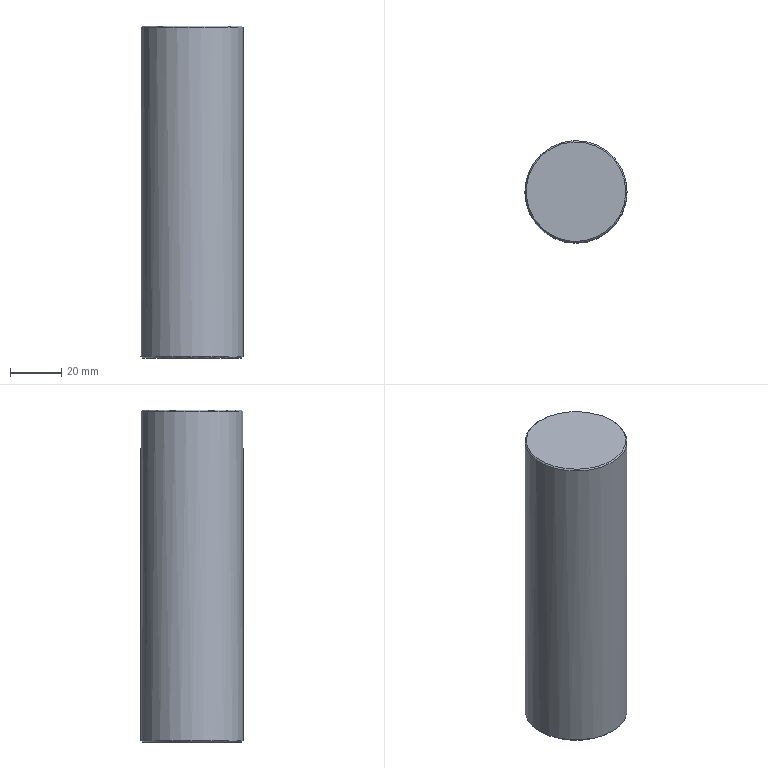Part | NX | features solid 2 | 1 solid | 7 faces | box 40 x 40 x 130 mm | volume 162539 mm3 | cone 3 | plane 2 | cylinder 2 | commonest cylinder face diameters 8 x1 40 x1
STEP:
#1=CARTESIAN_POINT('',(-74.5,-50.,-240.5));
#2=VERTEX_POINT('',#1);
#3=CARTESIAN_POINT('',(-55.,-50.,-240.5));
#4=DIRECTION('',(0.,0.,-1.));
#5=DIRECTION('',(-1.,0.,0.));
#6=AXIS2_PLACEMENT_3D('',#3,#4,#5);
#7=CIRCLE('',#6,19.5);
#8=EDGE_CURVE('',#2,#2,#7,.T.);
#9=ORIENTED_EDGE('',*,*,#8,.T.);
#10=EDGE_LOOP('',(#9));
#11=FACE_BOUND('',#10,.T.);
#12=CARTESIAN_POINT('',(-51.,-50.,-240.5));
#13=VERTEX_POINT('',#12);
#14=CARTESIAN_POINT('',(-55.,-50.,-240.5));
#15=DIRECTION('',(0.,0.,1.));
#16=DIRECTION('',(1.,0.,0.));
#17=AXIS2_PLACEMENT_3D('',#14,#15,#16);
#18=CIRCLE('',#17,4.);
#19=EDGE_CURVE('',#13,#13,#18,.T.);
#20=ORIENTED_EDGE('',*,*,#19,.T.);
#21=EDGE_LOOP('',(#20));
#22=FACE_BOUND('',#21,.T.);
#23=CARTESIAN_POINT('',(-55.,-50.,-240.5));
#24=DIRECTION('',(0.,0.,-1.));
#25=DIRECTION('',(-1.,0.,0.));
#26=AXIS2_PLACEMENT_3D('',#23,#24,#25);
#27=PLANE('',#26);
#28=ADVANCED_FACE('',(#11,#22),#27,.T.);
#29=CARTESIAN_POINT('',(-35.5,-50.,-110.5));
#30=VERTEX_POINT('',#29);
#31=CARTESIAN_POINT('',(-55.,-50.,-110.5));
#32=DIRECTION('',(0.,0.,1.));
#33=DIRECTION('',(1.,0.,0.));
#34=AXIS2_PLACEMENT_3D('',#31,#32,#33);
#35=CIRCLE('',#34,19.5);
#36=EDGE_CURVE('',#30,#30,#35,.T.);
#37=ORIENTED_EDGE('',*,*,#36,.T.);
#38=EDGE_LOOP('',(#37));
#39=FACE_BOUND('',#38,.T.);
#40=CARTESIAN_POINT('',(-55.,-50.,-110.5));
#41=DIRECTION('',(0.,0.,1.));
#42=DIRECTION('',(1.,0.,0.));
#43=AXIS2_PLACEMENT_3D('',#40,#41,#42);
#44=PLANE('',#43);
#45=ADVANCED_FACE('',(#39),#44,.T.);
#46=CARTESIAN_POINT('',(-75.,-50.,-240.));
#47=VERTEX_POINT('',#46);
#48=CARTESIAN_POINT('',(-55.,-50.,-240.));
#49=DIRECTION('',(0.,0.,-1.));
#50=DIRECTION('',(-1.,0.,0.));
#51=AXIS2_PLACEMENT_3D('',#48,#49,#50);
#52=CIRCLE('',#51,20.);
#53=EDGE_CURVE('',#47,#47,#52,.F.);
#54=ORIENTED_EDGE('',*,*,#53,.T.);
#55=EDGE_LOOP('',(#54));
#56=FACE_BOUND('',#55,.T.);
#57=CARTESIAN_POINT('',(-35.,-50.,-111.));
#58=VERTEX_POINT('',#57);
#59=CARTESIAN_POINT('',(-55.,-50.,-111.));
#60=DIRECTION('',(0.,0.,1.));
#61=DIRECTION('',(1.,0.,0.));
#62=AXIS2_PLACEMENT_3D('',#59,#60,#61);
#63=CIRCLE('',#62,20.);
#64=EDGE_CURVE('',#58,#58,#63,.F.);
#65=ORIENTED_EDGE('',*,*,#64,.T.);
#66=EDGE_LOOP('',(#65));
#67=FACE_BOUND('',#66,.T.);
#68=CARTESIAN_POINT('',(-55.,-50.,-110.5));
#69=DIRECTION('',(0.,0.,-1.));
#70=DIRECTION('',(1.,0.,0.));
#71=AXIS2_PLACEMENT_3D('',#68,#69,#70);
#72=CYLINDRICAL_SURFACE('',#71,20.);
#73=ADVANCED_FACE('',(#56,#67),#72,.T.);
#74=CARTESIAN_POINT('',(-51.,-50.,-225.5));
#75=VERTEX_POINT('',#74);
#76=CARTESIAN_POINT('',(-55.,-50.,-225.5));
#77=DIRECTION('',(0.,0.,1.));
#78=DIRECTION('',(1.,0.,0.));
#79=AXIS2_PLACEMENT_3D('',#76,#77,#78);
#80=CIRCLE('',#79,4.);
#81=EDGE_CURVE('',#75,#75,#80,.T.);
#82=ORIENTED_EDGE('',*,*,#81,.T.);
#83=EDGE_LOOP('',(#82));
#84=FACE_BOUND('',#83,.T.);
#85=ORIENTED_EDGE('',*,*,#19,.F.);
#86=EDGE_LOOP('',(#85));
#87=FACE_BOUND('',#86,.T.);
#88=CARTESIAN_POINT('',(-55.,-50.,-240.5));
#89=DIRECTION('',(0.,0.,1.));
#90=DIRECTION('',(1.,0.,0.));
#91=AXIS2_PLACEMENT_3D('',#88,#89,#90);
#92=CYLINDRICAL_SURFACE('',#91,4.);
#93=ADVANCED_FACE('',(#84,#87),#92,.F.);
#94=ORIENTED_EDGE('',*,*,#81,.F.);
#95=EDGE_LOOP('',(#94));
#96=FACE_BOUND('',#95,.T.);
#97=CARTESIAN_POINT('',(-55.,-50.,-223.19));
#98=VERTEX_POINT('',#97);
#99=VERTEX_LOOP('',#98);
#100=FACE_BOUND('',#99,.T.);
#101=CARTESIAN_POINT('',(-55.,-50.,-223.19));
#102=DIRECTION('',(0.,0.,-1.));
#103=DIRECTION('',(1.,0.,0.));
#104=AXIS2_PLACEMENT_3D('',#101,#102,#103);
#105=CONICAL_SURFACE('',#104,0.,1.047);
#106=ADVANCED_FACE('',(#96,#100),#105,.F.);
#107=ORIENTED_EDGE('',*,*,#8,.F.);
#108=EDGE_LOOP('',(#107));
#109=FACE_BOUND('',#108,.T.);
#110=ORIENTED_EDGE('',*,*,#53,.F.);
#111=EDGE_LOOP('',(#110));
#112=FACE_BOUND('',#111,.T.);
#113=CARTESIAN_POINT('',(-55.,-50.,-240.));
#114=DIRECTION('',(0.,0.,1.));
#115=DIRECTION('',(1.,0.,0.));
#116=AXIS2_PLACEMENT_3D('',#113,#114,#115);
#117=CONICAL_SURFACE('',#116,20.,0.7854);
#118=ADVANCED_FACE('',(#109,#112),#117,.T.);
#119=ORIENTED_EDGE('',*,*,#36,.F.);
#120=EDGE_LOOP('',(#119));
#121=FACE_BOUND('',#120,.T.);
#122=ORIENTED_EDGE('',*,*,#64,.F.);
#123=EDGE_LOOP('',(#122));
#124=FACE_BOUND('',#123,.T.);
#125=CARTESIAN_POINT('',(-55.,-50.,-111.));
#126=DIRECTION('',(0.,0.,-1.));
#127=DIRECTION('',(-1.,0.,0.));
#128=AXIS2_PLACEMENT_3D('',#125,#126,#127);
#129=CONICAL_SURFACE('',#128,20.,0.7854);
#130=ADVANCED_FACE('',(#121,#124),#129,.T.);
#131=CLOSED_SHELL('',(#28,#45,#73,#93,#106,#118,#130));
#132=MANIFOLD_SOLID_BREP('',#131);
#133=(LENGTH_UNIT()NAMED_UNIT(*)SI_UNIT(.MILLI.,.METRE.));
#134=UNCERTAINTY_MEASURE_WITH_UNIT(LENGTH_MEASURE(0.00001),#133,'','');
#135=(NAMED_UNIT(*)PLANE_ANGLE_UNIT()SI_UNIT($,.RADIAN.));
#136=(NAMED_UNIT(*)SI_UNIT($,.STERADIAN.)SOLID_ANGLE_UNIT());
#137=(GEOMETRIC_REPRESENTATION_CONTEXT(3)GLOBAL_UNCERTAINTY_ASSIGNED_CONTEXT((#134))GLOBAL_UNIT_ASSIGNED_CONTEXT((#133,#135,#136))REPRESENTATION_CONTEXT('',''));
#138=ADVANCED_BREP_SHAPE_REPRESENTATION('',(#132),#137);